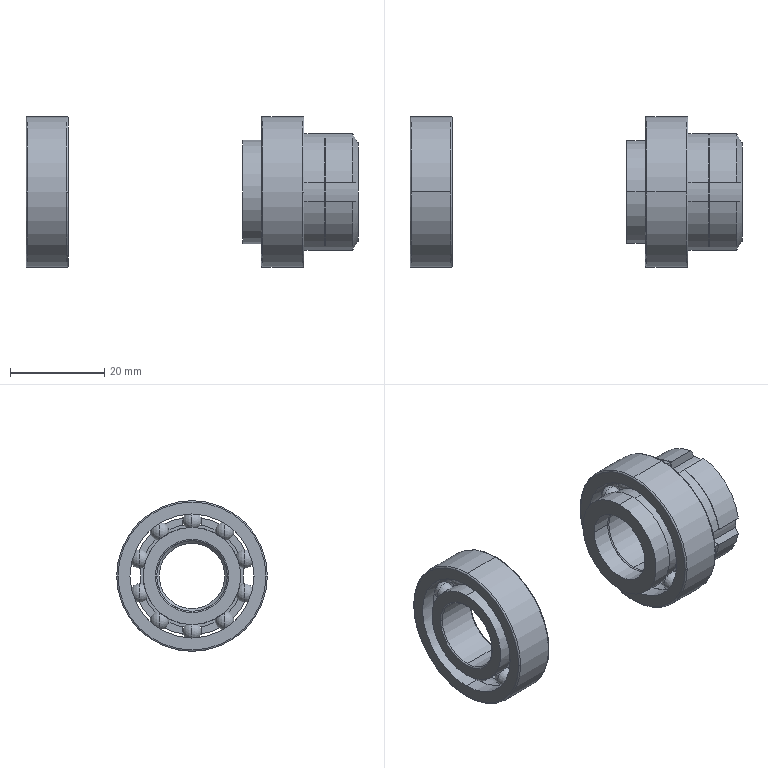Part | NX | 4 solids | 241 faces | box 70.5 x 32 x 32 mm | volume 12073 mm3 | torus 82 | cylinder 52 | plane 47 | sphere 40 | cone 20 | commonest cylinder face diameters 20.667 x8 21 x8 25 x8 26.333 x8 13.917 x4 15 x4